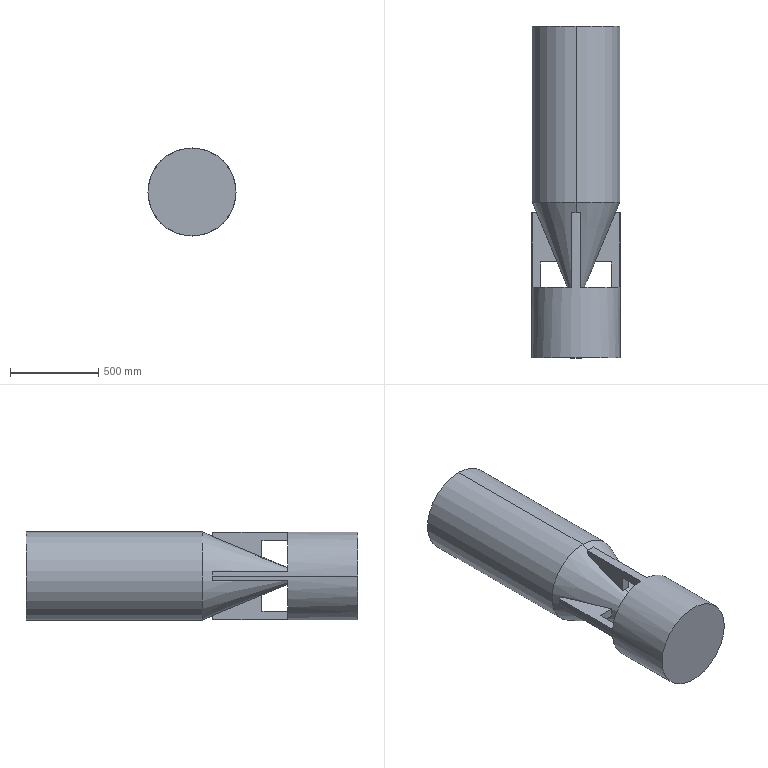Part | SolidWorks | features ICE 3, Revolution 2, Shell 1 | 2 solids | 37 faces | box 500 x 1885 x 500 mm | volume 205239805 mm3 | plane 27 | cylinder 6 | cone 4 | commonest cylinder face diameters 500 x4 360 x2